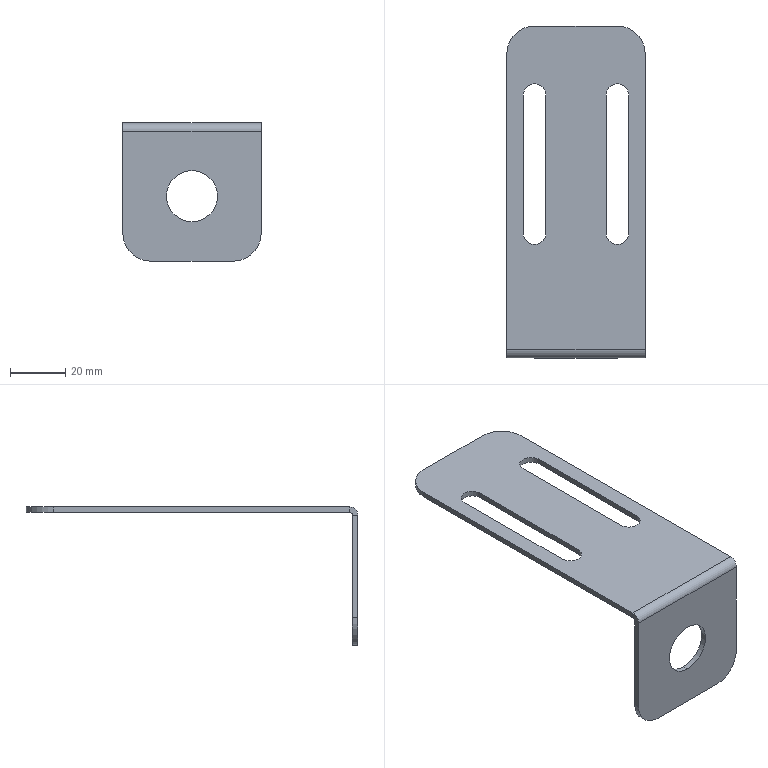Part | SolidWorks | features ICE 2, Fillet 1, FlatPattern 1, SMBaseFlange 1, SheetMetal 1 | 1 solid | 28 faces | box 50 x 120 x 50 mm | volume 14154 mm3 | plane 16 | cylinder 12 | commonest cylinder face diameters 8.2 x4 20 x4 18.5 x2 2 x1 6 x1
STEP:
#1=CARTESIAN_POINT('',(0.,0.,-35.75));
#2=VERTEX_POINT('',#1);
#3=CARTESIAN_POINT('',(0.,0.,-17.25));
#4=VERTEX_POINT('',#3);
#5=CARTESIAN_POINT('',(0.,0.,-26.5));
#6=DIRECTION('',(0.,1.,0.));
#7=DIRECTION('',(0.,0.,-1.));
#8=AXIS2_PLACEMENT_3D('',#5,#6,#7);
#9=CIRCLE('',#8,9.25);
#10=EDGE_CURVE('',#2,#4,#9,.T.);
#11=ORIENTED_EDGE('',*,*,#10,.F.);
#12=CARTESIAN_POINT('',(0.,2.,-35.75));
#13=VERTEX_POINT('',#12);
#14=CARTESIAN_POINT('',(0.,-0.001,-35.75));
#15=DIRECTION('',(0.,1.,0.));
#16=VECTOR('',#15,1000.);
#17=LINE('',#14,#16);
#18=EDGE_CURVE('',#2,#13,#17,.T.);
#19=ORIENTED_EDGE('',*,*,#18,.T.);
#20=CARTESIAN_POINT('',(0.,2.,-17.25));
#21=VERTEX_POINT('',#20);
#22=CARTESIAN_POINT('',(0.,2.,-26.5));
#23=DIRECTION('',(0.,1.,0.));
#24=DIRECTION('',(0.,0.,1.));
#25=AXIS2_PLACEMENT_3D('',#22,#23,#24);
#26=CIRCLE('',#25,9.25);
#27=EDGE_CURVE('',#13,#21,#26,.T.);
#28=ORIENTED_EDGE('',*,*,#27,.T.);
#29=CARTESIAN_POINT('',(0.,-0.001,-17.25));
#30=DIRECTION('',(0.,1.,0.));
#31=VECTOR('',#30,1000.);
#32=LINE('',#29,#31);
#33=EDGE_CURVE('',#4,#21,#32,.T.);
#34=ORIENTED_EDGE('',*,*,#33,.F.);
#35=EDGE_LOOP('',(#11,#19,#28,#34));
#36=FACE_OUTER_BOUND('',#35,.T.);
#37=CARTESIAN_POINT('',(0.,-0.001,-26.5));
#38=DIRECTION('',(0.,1.,0.));
#39=DIRECTION('',(0.,0.,1.));
#40=AXIS2_PLACEMENT_3D('',#37,#38,#39);
#41=CYLINDRICAL_SURFACE('',#40,9.25);
#42=ADVANCED_FACE('',(#36),#41,.F.);
#43=CARTESIAN_POINT('',(25.,3.,0.));
#44=VERTEX_POINT('',#43);
#45=CARTESIAN_POINT('',(25.,3.,-2.));
#46=VERTEX_POINT('',#45);
#47=CARTESIAN_POINT('',(25.,3.,0.));
#48=DIRECTION('',(0.,0.,-1.));
#49=VECTOR('',#48,1000.);
#50=LINE('',#47,#49);
#51=EDGE_CURVE('',#44,#46,#50,.T.);
#52=ORIENTED_EDGE('',*,*,#51,.F.);
#53=CARTESIAN_POINT('',(25.,0.,-3.));
#54=VERTEX_POINT('',#53);
#55=CARTESIAN_POINT('',(25.,3.,-3.));
#56=DIRECTION('',(-1.,0.,0.));
#57=DIRECTION('',(0.,0.,-1.));
#58=AXIS2_PLACEMENT_3D('',#55,#56,#57);
#59=CIRCLE('',#58,3.);
#60=EDGE_CURVE('',#54,#44,#59,.T.);
#61=ORIENTED_EDGE('',*,*,#60,.F.);
#62=CARTESIAN_POINT('',(25.,2.,-3.));
#63=VERTEX_POINT('',#62);
#64=CARTESIAN_POINT('',(25.,2.,-3.));
#65=DIRECTION('',(0.,-1.,0.));
#66=VECTOR('',#65,1000.);
#67=LINE('',#64,#66);
#68=EDGE_CURVE('',#63,#54,#67,.T.);
#69=ORIENTED_EDGE('',*,*,#68,.F.);
#70=CARTESIAN_POINT('',(25.,3.,-3.));
#71=DIRECTION('',(-1.,0.,0.));
#72=DIRECTION('',(0.,0.,-1.));
#73=AXIS2_PLACEMENT_3D('',#70,#71,#72);
#74=CIRCLE('',#73,1.);
#75=EDGE_CURVE('',#63,#46,#74,.T.);
#76=ORIENTED_EDGE('',*,*,#75,.T.);
#77=EDGE_LOOP('',(#52,#61,#69,#76));
#78=FACE_OUTER_BOUND('',#77,.T.);
#79=CARTESIAN_POINT('',(25.,3.,0.));
#80=DIRECTION('',(1.,0.,0.));
#81=DIRECTION('',(0.,0.,-1.));
#82=AXIS2_PLACEMENT_3D('',#79,#80,#81);
#83=PLANE('',#82);
#84=ADVANCED_FACE('',(#78),#83,.T.);
#85=CARTESIAN_POINT('',(25.,110.,-2.));
#86=VERTEX_POINT('',#85);
#87=CARTESIAN_POINT('',(25.,0.,-2.));
#88=DIRECTION('',(0.,1.,0.));
#89=VECTOR('',#88,1000.);
#90=LINE('',#87,#89);
#91=EDGE_CURVE('',#46,#86,#90,.T.);
#92=ORIENTED_EDGE('',*,*,#91,.T.);
#93=CARTESIAN_POINT('',(25.,110.,0.));
#94=VERTEX_POINT('',#93);
#95=CARTESIAN_POINT('',(25.,110.,-3.));
#96=DIRECTION('',(0.,0.,1.));
#97=VECTOR('',#96,1000.);
#98=LINE('',#95,#97);
#99=EDGE_CURVE('',#86,#94,#98,.T.);
#100=ORIENTED_EDGE('',*,*,#99,.T.);
#101=CARTESIAN_POINT('',(25.,0.,0.));
#102=DIRECTION('',(0.,1.,0.));
#103=VECTOR('',#102,1000.);
#104=LINE('',#101,#103);
#105=EDGE_CURVE('',#44,#94,#104,.T.);
#106=ORIENTED_EDGE('',*,*,#105,.F.);
#107=ORIENTED_EDGE('',*,*,#51,.T.);
#108=EDGE_LOOP('',(#92,#100,#106,#107));
#109=FACE_OUTER_BOUND('',#108,.T.);
#110=CARTESIAN_POINT('',(25.,2.,-3.));
#111=DIRECTION('',(1.,0.,0.));
#112=DIRECTION('',(0.,0.,-1.));
#113=AXIS2_PLACEMENT_3D('',#110,#111,#112);
#114=PLANE('',#113);
#115=ADVANCED_FACE('',(#109),#114,.T.);
#116=CARTESIAN_POINT('',(-25.,0.,-3.));
#117=VERTEX_POINT('',#116);
#118=CARTESIAN_POINT('',(-25.,2.,-3.));
#119=VERTEX_POINT('',#118);
#120=CARTESIAN_POINT('',(-25.,0.,-3.));
#121=DIRECTION('',(0.,1.,0.));
#122=VECTOR('',#121,1000.);
#123=LINE('',#120,#122);
#124=EDGE_CURVE('',#117,#119,#123,.T.);
#125=ORIENTED_EDGE('',*,*,#124,.F.);
#126=CARTESIAN_POINT('',(-25.,3.,0.));
#127=VERTEX_POINT('',#126);
#128=CARTESIAN_POINT('',(-25.,3.,-3.));
#129=DIRECTION('',(-1.,0.,0.));
#130=DIRECTION('',(0.,0.,-1.));
#131=AXIS2_PLACEMENT_3D('',#128,#129,#130);
#132=CIRCLE('',#131,3.);
#133=EDGE_CURVE('',#117,#127,#132,.T.);
#134=ORIENTED_EDGE('',*,*,#133,.T.);
#135=CARTESIAN_POINT('',(-25.,3.,-2.));
#136=VERTEX_POINT('',#135);
#137=CARTESIAN_POINT('',(-25.,3.,-2.));
#138=DIRECTION('',(0.,0.,1.));
#139=VECTOR('',#138,1000.);
#140=LINE('',#137,#139);
#141=EDGE_CURVE('',#136,#127,#140,.T.);
#142=ORIENTED_EDGE('',*,*,#141,.F.);
#143=CARTESIAN_POINT('',(-25.,3.,-3.));
#144=DIRECTION('',(-1.,0.,0.));
#145=DIRECTION('',(0.,0.,-1.));
#146=AXIS2_PLACEMENT_3D('',#143,#144,#145);
#147=CIRCLE('',#146,1.);
#148=EDGE_CURVE('',#119,#136,#147,.T.);
#149=ORIENTED_EDGE('',*,*,#148,.F.);
#150=EDGE_LOOP('',(#125,#134,#142,#149));
#151=FACE_OUTER_BOUND('',#150,.T.);
#152=CARTESIAN_POINT('',(-25.,0.,-3.));
#153=DIRECTION('',(-1.,0.,0.));
#154=DIRECTION('',(0.,0.,1.));
#155=AXIS2_PLACEMENT_3D('',#152,#153,#154);
#156=PLANE('',#155);
#157=ADVANCED_FACE('',(#151),#156,.T.);
#158=CARTESIAN_POINT('',(-25.,2.,-40.));
#159=VERTEX_POINT('',#158);
#160=CARTESIAN_POINT('',(-25.,2.,0.));
#161=DIRECTION('',(0.,0.,1.));
#162=VECTOR('',#161,1000.);
#163=LINE('',#160,#162);
#164=EDGE_CURVE('',#159,#119,#163,.T.);
#165=ORIENTED_EDGE('',*,*,#164,.F.);
#166=CARTESIAN_POINT('',(-25.,0.,-40.));
#167=VERTEX_POINT('',#166);
#168=CARTESIAN_POINT('',(-25.,3.,-40.));
#169=DIRECTION('',(0.,-1.,0.));
#170=VECTOR('',#169,1000.);
#171=LINE('',#168,#170);
#172=EDGE_CURVE('',#159,#167,#171,.T.);
#173=ORIENTED_EDGE('',*,*,#172,.T.);
#174=CARTESIAN_POINT('',(-25.,0.,0.));
#175=DIRECTION('',(0.,0.,1.));
#176=VECTOR('',#175,1000.);
#177=LINE('',#174,#176);
#178=EDGE_CURVE('',#167,#117,#177,.T.);
#179=ORIENTED_EDGE('',*,*,#178,.T.);
#180=ORIENTED_EDGE('',*,*,#124,.T.);
#181=EDGE_LOOP('',(#165,#173,#179,#180));
#182=FACE_OUTER_BOUND('',#181,.T.);
#183=CARTESIAN_POINT('',(-25.,3.,-2.));
#184=DIRECTION('',(-1.,0.,0.));
#185=DIRECTION('',(0.,0.,1.));
#186=AXIS2_PLACEMENT_3D('',#183,#184,#185);
#187=PLANE('',#186);
#188=ADVANCED_FACE('',(#182),#187,.T.);
#189=CARTESIAN_POINT('',(-19.1,45.,-2.));
#190=VERTEX_POINT('',#189);
#191=CARTESIAN_POINT('',(-19.1,95.,-2.));
#192=VERTEX_POINT('',#191);
#193=CARTESIAN_POINT('',(-19.1,45.,-2.));
#194=DIRECTION('',(0.,1.,0.));
#195=VECTOR('',#194,1000.);
#196=LINE('',#193,#195);
#197=EDGE_CURVE('',#190,#192,#196,.T.);
#198=ORIENTED_EDGE('',*,*,#197,.F.);
#199=CARTESIAN_POINT('',(-10.9,45.,-2.));
#200=VERTEX_POINT('',#199);
#201=CARTESIAN_POINT('',(-15.,45.,-2.));
#202=DIRECTION('',(0.,0.,-1.));
#203=DIRECTION('',(-1.,0.,0.));
#204=AXIS2_PLACEMENT_3D('',#201,#202,#203);
#205=CIRCLE('',#204,4.1);
#206=EDGE_CURVE('',#200,#190,#205,.T.);
#207=ORIENTED_EDGE('',*,*,#206,.F.);
#208=CARTESIAN_POINT('',(-10.9,95.,-2.));
#209=VERTEX_POINT('',#208);
#210=CARTESIAN_POINT('',(-10.9,45.,-2.));
#211=DIRECTION('',(0.,-1.,0.));
#212=VECTOR('',#211,1000.);
#213=LINE('',#210,#212);
#214=EDGE_CURVE('',#209,#200,#213,.T.);
#215=ORIENTED_EDGE('',*,*,#214,.F.);
#216=CARTESIAN_POINT('',(-15.,95.,-2.));
#217=DIRECTION('',(0.,0.,-1.));
#218=DIRECTION('',(-1.,0.,0.));
#219=AXIS2_PLACEMENT_3D('',#216,#217,#218);
#220=CIRCLE('',#219,4.1);
#221=EDGE_CURVE('',#192,#209,#220,.T.);
#222=ORIENTED_EDGE('',*,*,#221,.F.);
#223=EDGE_LOOP('',(#198,#207,#215,#222));
#224=FACE_BOUND('',#223,.T.);
#225=CARTESIAN_POINT('',(10.9,45.,-2.));
#226=VERTEX_POINT('',#225);
#227=CARTESIAN_POINT('',(10.9,95.,-2.));
#228=VERTEX_POINT('',#227);
#229=CARTESIAN_POINT('',(10.9,45.,-2.));
#230=DIRECTION('',(0.,1.,0.));
#231=VECTOR('',#230,1000.);
#232=LINE('',#229,#231);
#233=EDGE_CURVE('',#226,#228,#232,.T.);
#234=ORIENTED_EDGE('',*,*,#233,.F.);
#235=CARTESIAN_POINT('',(19.1,45.,-2.));
#236=VERTEX_POINT('',#235);
#237=CARTESIAN_POINT('',(15.,45.,-2.));
#238=DIRECTION('',(0.,0.,-1.));
#239=DIRECTION('',(1.,0.,0.));
#240=AXIS2_PLACEMENT_3D('',#237,#238,#239);
#241=CIRCLE('',#240,4.1);
#242=EDGE_CURVE('',#236,#226,#241,.T.);
#243=ORIENTED_EDGE('',*,*,#242,.F.);
#244=CARTESIAN_POINT('',(19.1,95.,-2.));
#245=VERTEX_POINT('',#244);
#246=CARTESIAN_POINT('',(19.1,45.,-2.));
#247=DIRECTION('',(0.,-1.,0.));
#248=VECTOR('',#247,1000.);
#249=LINE('',#246,#248);
#250=EDGE_CURVE('',#245,#236,#249,.T.);
#251=ORIENTED_EDGE('',*,*,#250,.F.);
#252=CARTESIAN_POINT('',(15.,95.,-2.));
#253=DIRECTION('',(0.,0.,-1.));
#254=DIRECTION('',(1.,0.,0.));
#255=AXIS2_PLACEMENT_3D('',#252,#253,#254);
#256=CIRCLE('',#255,4.1);
#257=EDGE_CURVE('',#228,#245,#256,.T.);
#258=ORIENTED_EDGE('',*,*,#257,.F.);
#259=EDGE_LOOP('',(#234,#243,#251,#258));
#260=FACE_BOUND('',#259,.T.);
#261=CARTESIAN_POINT('',(15.,120.,-2.));
#262=VERTEX_POINT('',#261);
#263=CARTESIAN_POINT('',(-15.,120.,-2.));
#264=VERTEX_POINT('',#263);
#265=CARTESIAN_POINT('',(25.,120.,-2.));
#266=DIRECTION('',(-1.,0.,0.));
#267=VECTOR('',#266,1000.);
#268=LINE('',#265,#267);
#269=EDGE_CURVE('',#262,#264,#268,.T.);
#270=ORIENTED_EDGE('',*,*,#269,.F.);
#271=CARTESIAN_POINT('',(15.,110.,-2.));
#272=DIRECTION('',(0.,0.,-1.));
#273=DIRECTION('',(1.,0.,0.));
#274=AXIS2_PLACEMENT_3D('',#271,#272,#273);
#275=CIRCLE('',#274,10.);
#276=EDGE_CURVE('',#262,#86,#275,.T.);
#277=ORIENTED_EDGE('',*,*,#276,.T.);
#278=ORIENTED_EDGE('',*,*,#91,.F.);
#279=CARTESIAN_POINT('',(25.,3.,-2.));
#280=DIRECTION('',(-1.,0.,0.));
#281=VECTOR('',#280,1000.);
#282=LINE('',#279,#281);
#283=EDGE_CURVE('',#46,#136,#282,.T.);
#284=ORIENTED_EDGE('',*,*,#283,.T.);
#285=CARTESIAN_POINT('',(-25.,110.,-2.));
#286=VERTEX_POINT('',#285);
#287=CARTESIAN_POINT('',(-25.,0.,-2.));
#288=DIRECTION('',(0.,1.,0.));
#289=VECTOR('',#288,1000.);
#290=LINE('',#287,#289);
#291=EDGE_CURVE('',#136,#286,#290,.T.);
#292=ORIENTED_EDGE('',*,*,#291,.T.);
#293=CARTESIAN_POINT('',(-15.,110.,-2.));
#294=DIRECTION('',(0.,0.,-1.));
#295=DIRECTION('',(1.,0.,0.));
#296=AXIS2_PLACEMENT_3D('',#293,#294,#295);
#297=CIRCLE('',#296,10.);
#298=EDGE_CURVE('',#286,#264,#297,.T.);
#299=ORIENTED_EDGE('',*,*,#298,.T.);
#300=EDGE_LOOP('',(#270,#277,#278,#284,#292,#299));
#301=FACE_OUTER_BOUND('',#300,.T.);
#302=CARTESIAN_POINT('',(25.,0.,-2.));
#303=DIRECTION('',(0.,0.,1.));
#304=DIRECTION('',(1.,0.,0.));
#305=AXIS2_PLACEMENT_3D('',#302,#303,#304);
#306=PLANE('',#305);
#307=ADVANCED_FACE('',(#224,#260,#301),#306,.F.);
#308=CARTESIAN_POINT('',(15.,120.,0.));
#309=VERTEX_POINT('',#308);
#310=CARTESIAN_POINT('',(-15.,120.,0.));
#311=VERTEX_POINT('',#310);
#312=CARTESIAN_POINT('',(25.,120.,0.));
#313=DIRECTION('',(-1.,0.,0.));
#314=VECTOR('',#313,1000.);
#315=LINE('',#312,#314);
#316=EDGE_CURVE('',#309,#311,#315,.T.);
#317=ORIENTED_EDGE('',*,*,#316,.F.);
#318=CARTESIAN_POINT('',(15.,120.,0.));
#319=DIRECTION('',(0.,0.,-1.));
#320=VECTOR('',#319,1000.);
#321=LINE('',#318,#320);
#322=EDGE_CURVE('',#309,#262,#321,.T.);
#323=ORIENTED_EDGE('',*,*,#322,.T.);
#324=ORIENTED_EDGE('',*,*,#269,.T.);
#325=CARTESIAN_POINT('',(-15.,120.,0.));
#326=DIRECTION('',(0.,0.,1.));
#327=VECTOR('',#326,1000.);
#328=LINE('',#325,#327);
#329=EDGE_CURVE('',#264,#311,#328,.T.);
#330=ORIENTED_EDGE('',*,*,#329,.T.);
#331=EDGE_LOOP('',(#317,#323,#324,#330));
#332=FACE_OUTER_BOUND('',#331,.T.);
#333=CARTESIAN_POINT('',(25.,120.,0.));
#334=DIRECTION('',(0.,1.,0.));
#335=DIRECTION('',(0.,0.,1.));
#336=AXIS2_PLACEMENT_3D('',#333,#334,#335);
#337=PLANE('',#336);
#338=ADVANCED_FACE('',(#332),#337,.T.);
#339=CARTESIAN_POINT('',(-10.9,45.,0.));
#340=VERTEX_POINT('',#339);
#341=CARTESIAN_POINT('',(-19.1,45.,0.));
#342=VERTEX_POINT('',#341);
#343=CARTESIAN_POINT('',(-15.,45.,0.));
#344=DIRECTION('',(0.,0.,-1.));
#345=DIRECTION('',(1.,0.,0.));
#346=AXIS2_PLACEMENT_3D('',#343,#344,#345);
#347=CIRCLE('',#346,4.1);
#348=EDGE_CURVE('',#340,#342,#347,.T.);
#349=ORIENTED_EDGE('',*,*,#348,.T.);
#350=CARTESIAN_POINT('',(-19.1,95.,0.));
#351=VERTEX_POINT('',#350);
#352=CARTESIAN_POINT('',(-19.1,45.,0.));
#353=DIRECTION('',(0.,1.,0.));
#354=VECTOR('',#353,1000.);
#355=LINE('',#352,#354);
#356=EDGE_CURVE('',#342,#351,#355,.T.);
#357=ORIENTED_EDGE('',*,*,#356,.T.);
#358=CARTESIAN_POINT('',(-10.9,95.,0.));
#359=VERTEX_POINT('',#358);
#360=CARTESIAN_POINT('',(-15.,95.,0.));
#361=DIRECTION('',(0.,0.,-1.));
#362=DIRECTION('',(1.,0.,0.));
#363=AXIS2_PLACEMENT_3D('',#360,#361,#362);
#364=CIRCLE('',#363,4.1);
#365=EDGE_CURVE('',#351,#359,#364,.T.);
#366=ORIENTED_EDGE('',*,*,#365,.T.);
#367=CARTESIAN_POINT('',(-10.9,45.,0.));
#368=DIRECTION('',(0.,-1.,0.));
#369=VECTOR('',#368,1000.);
#370=LINE('',#367,#369);
#371=EDGE_CURVE('',#359,#340,#370,.T.);
#372=ORIENTED_EDGE('',*,*,#371,.T.);
#373=EDGE_LOOP('',(#349,#357,#366,#372));
#374=FACE_BOUND('',#373,.T.);
#375=CARTESIAN_POINT('',(19.1,45.,0.));
#376=VERTEX_POINT('',#375);
#377=CARTESIAN_POINT('',(10.9,45.,0.));
#378=VERTEX_POINT('',#377);
#379=CARTESIAN_POINT('',(15.,45.,0.));
#380=DIRECTION('',(0.,0.,-1.));
#381=DIRECTION('',(1.,0.,0.));
#382=AXIS2_PLACEMENT_3D('',#379,#380,#381);
#383=CIRCLE('',#382,4.1);
#384=EDGE_CURVE('',#376,#378,#383,.T.);
#385=ORIENTED_EDGE('',*,*,#384,.T.);
#386=CARTESIAN_POINT('',(10.9,95.,0.));
#387=VERTEX_POINT('',#386);
#388=CARTESIAN_POINT('',(10.9,45.,0.));
#389=DIRECTION('',(0.,1.,0.));
#390=VECTOR('',#389,1000.);
#391=LINE('',#388,#390);
#392=EDGE_CURVE('',#378,#387,#391,.T.);
#393=ORIENTED_EDGE('',*,*,#392,.T.);
#394=CARTESIAN_POINT('',(19.1,95.,0.));
#395=VERTEX_POINT('',#394);
#396=CARTESIAN_POINT('',(15.,95.,0.));
#397=DIRECTION('',(0.,0.,-1.));
#398=DIRECTION('',(1.,0.,0.));
#399=AXIS2_PLACEMENT_3D('',#396,#397,#398);
#400=CIRCLE('',#399,4.1);
#401=EDGE_CURVE('',#387,#395,#400,.T.);
#402=ORIENTED_EDGE('',*,*,#401,.T.);
#403=CARTESIAN_POINT('',(19.1,45.,0.));
#404=DIRECTION('',(0.,-1.,0.));
#405=VECTOR('',#404,1000.);
#406=LINE('',#403,#405);
#407=EDGE_CURVE('',#395,#376,#406,.T.);
#408=ORIENTED_EDGE('',*,*,#407,.T.);
#409=EDGE_LOOP('',(#385,#393,#402,#408));
#410=FACE_BOUND('',#409,.T.);
#411=ORIENTED_EDGE('',*,*,#105,.T.);
#412=CARTESIAN_POINT('',(15.,110.,0.));
#413=DIRECTION('',(0.,0.,1.));
#414=DIRECTION('',(1.,0.,0.));
#415=AXIS2_PLACEMENT_3D('',#412,#413,#414);
#416=CIRCLE('',#415,10.);
#417=EDGE_CURVE('',#94,#309,#416,.T.);
#418=ORIENTED_EDGE('',*,*,#417,.T.);
#419=ORIENTED_EDGE('',*,*,#316,.T.);
#420=CARTESIAN_POINT('',(-25.,110.,0.));
#421=VERTEX_POINT('',#420);
#422=CARTESIAN_POINT('',(-15.,110.,0.));
#423=DIRECTION('',(0.,0.,1.));
#424=DIRECTION('',(1.,0.,0.));
#425=AXIS2_PLACEMENT_3D('',#422,#423,#424);
#426=CIRCLE('',#425,10.);
#427=EDGE_CURVE('',#311,#421,#426,.T.);
#428=ORIENTED_EDGE('',*,*,#427,.T.);
#429=CARTESIAN_POINT('',(-25.,0.,0.));
#430=DIRECTION('',(0.,1.,0.));
#431=VECTOR('',#430,1000.);
#432=LINE('',#429,#431);
#433=EDGE_CURVE('',#127,#421,#432,.T.);
#434=ORIENTED_EDGE('',*,*,#433,.F.);
#435=CARTESIAN_POINT('',(25.,3.,0.));
#436=DIRECTION('',(-1.,0.,0.));
#437=VECTOR('',#436,1000.);
#438=LINE('',#435,#437);
#439=EDGE_CURVE('',#44,#127,#438,.T.);
#440=ORIENTED_EDGE('',*,*,#439,.F.);
#441=EDGE_LOOP('',(#411,#418,#419,#428,#434,#440));
#442=FACE_OUTER_BOUND('',#441,.T.);
#443=CARTESIAN_POINT('',(25.,0.,0.));
#444=DIRECTION('',(0.,0.,1.));
#445=DIRECTION('',(1.,0.,0.));
#446=AXIS2_PLACEMENT_3D('',#443,#444,#445);
#447=PLANE('',#446);
#448=ADVANCED_FACE('',(#374,#410,#442),#447,.T.);
#449=ORIENTED_EDGE('',*,*,#133,.F.);
#450=CARTESIAN_POINT('',(25.,0.,-3.));
#451=DIRECTION('',(-1.,0.,0.));
#452=VECTOR('',#451,1000.);
#453=LINE('',#450,#452);
#454=EDGE_CURVE('',#54,#117,#453,.T.);
#455=ORIENTED_EDGE('',*,*,#454,.F.);
#456=ORIENTED_EDGE('',*,*,#60,.T.);
#457=ORIENTED_EDGE('',*,*,#439,.T.);
#458=EDGE_LOOP('',(#449,#455,#456,#457));
#459=FACE_OUTER_BOUND('',#458,.T.);
#460=CARTESIAN_POINT('',(25.,3.,-3.));
#461=DIRECTION('',(-1.,0.,0.));
#462=DIRECTION('',(0.,0.,1.));
#463=AXIS2_PLACEMENT_3D('',#460,#461,#462);
#464=CYLINDRICAL_SURFACE('',#463,3.);
#465=ADVANCED_FACE('',(#459),#464,.T.);
#466=CARTESIAN_POINT('',(0.,0.,-26.5));
#467=DIRECTION('',(0.,1.,0.));
#468=DIRECTION('',(0.,0.,-1.));
#469=AXIS2_PLACEMENT_3D('',#466,#467,#468);
#470=CIRCLE('',#469,9.25);
#471=EDGE_CURVE('',#4,#2,#470,.T.);
#472=ORIENTED_EDGE('',*,*,#471,.T.);
#473=ORIENTED_EDGE('',*,*,#10,.T.);
#474=EDGE_LOOP('',(#472,#473));
#475=FACE_BOUND('',#474,.T.);
#476=CARTESIAN_POINT('',(15.,0.,-50.));
#477=VERTEX_POINT('',#476);
#478=CARTESIAN_POINT('',(-15.,0.,-50.));
#479=VERTEX_POINT('',#478);
#480=CARTESIAN_POINT('',(25.,0.,-50.));
#481=DIRECTION('',(-1.,0.,0.));
#482=VECTOR('',#481,1000.);
#483=LINE('',#480,#482);
#484=EDGE_CURVE('',#477,#479,#483,.T.);
#485=ORIENTED_EDGE('',*,*,#484,.F.);
#486=CARTESIAN_POINT('',(25.,0.,-40.));
#487=VERTEX_POINT('',#486);
#488=CARTESIAN_POINT('',(15.,0.,-40.));
#489=DIRECTION('',(0.,-1.,0.));
#490=DIRECTION('',(0.,0.,-1.));
#491=AXIS2_PLACEMENT_3D('',#488,#489,#490);
#492=CIRCLE('',#491,10.);
#493=EDGE_CURVE('',#477,#487,#492,.T.);
#494=ORIENTED_EDGE('',*,*,#493,.T.);
#495=CARTESIAN_POINT('',(25.,0.,0.));
#496=DIRECTION('',(0.,0.,1.));
#497=VECTOR('',#496,1000.);
#498=LINE('',#495,#497);
#499=EDGE_CURVE('',#487,#54,#498,.T.);
#500=ORIENTED_EDGE('',*,*,#499,.T.);
#501=ORIENTED_EDGE('',*,*,#454,.T.);
#502=ORIENTED_EDGE('',*,*,#178,.F.);
#503=CARTESIAN_POINT('',(-15.,0.,-40.));
#504=DIRECTION('',(0.,-1.,0.));
#505=DIRECTION('',(0.,0.,-1.));
#506=AXIS2_PLACEMENT_3D('',#503,#504,#505);
#507=CIRCLE('',#506,10.);
#508=EDGE_CURVE('',#167,#479,#507,.T.);
#509=ORIENTED_EDGE('',*,*,#508,.T.);
#510=EDGE_LOOP('',(#485,#494,#500,#501,#502,#509));
#511=FACE_OUTER_BOUND('',#510,.T.);
#512=CARTESIAN_POINT('',(25.,0.,0.));
#513=DIRECTION('',(0.,-1.,0.));
#514=DIRECTION('',(0.,0.,-1.));
#515=AXIS2_PLACEMENT_3D('',#512,#513,#514);
#516=PLANE('',#515);
#517=ADVANCED_FACE('',(#475,#511),#516,.T.);
#518=CARTESIAN_POINT('',(15.,2.,-50.));
#519=VERTEX_POINT('',#518);
#520=CARTESIAN_POINT('',(-15.,2.,-50.));
#521=VERTEX_POINT('',#520);
#522=CARTESIAN_POINT('',(25.,2.,-50.));
#523=DIRECTION('',(-1.,0.,0.));
#524=VECTOR('',#523,1000.);
#525=LINE('',#522,#524);
#526=EDGE_CURVE('',#519,#521,#525,.T.);
#527=ORIENTED_EDGE('',*,*,#526,.F.);
#528=CARTESIAN_POINT('',(15.,2.,-50.));
#529=DIRECTION('',(0.,-1.,0.));
#530=VECTOR('',#529,1000.);
#531=LINE('',#528,#530);
#532=EDGE_CURVE('',#519,#477,#531,.T.);
#533=ORIENTED_EDGE('',*,*,#532,.T.);
#534=ORIENTED_EDGE('',*,*,#484,.T.);
#535=CARTESIAN_POINT('',(-15.,2.,-50.));
#536=DIRECTION('',(0.,1.,0.));
#537=VECTOR('',#536,1000.);
#538=LINE('',#535,#537);
#539=EDGE_CURVE('',#479,#521,#538,.T.);
#540=ORIENTED_EDGE('',*,*,#539,.T.);
#541=EDGE_LOOP('',(#527,#533,#534,#540));
#542=FACE_OUTER_BOUND('',#541,.T.);
#543=CARTESIAN_POINT('',(25.,2.,-50.));
#544=DIRECTION('',(0.,0.,-1.));
#545=DIRECTION('',(-1.,0.,0.));
#546=AXIS2_PLACEMENT_3D('',#543,#544,#545);
#547=PLANE('',#546);
#548=ADVANCED_FACE('',(#542),#547,.T.);
#549=CARTESIAN_POINT('',(0.,2.,-26.5));
#550=DIRECTION('',(0.,1.,0.));
#551=DIRECTION('',(0.,0.,1.));
#552=AXIS2_PLACEMENT_3D('',#549,#550,#551);
#553=CIRCLE('',#552,9.25);
#554=EDGE_CURVE('',#21,#13,#553,.T.);
#555=ORIENTED_EDGE('',*,*,#554,.F.);
#556=ORIENTED_EDGE('',*,*,#27,.F.);
#557=EDGE_LOOP('',(#555,#556));
#558=FACE_BOUND('',#557,.T.);
#559=CARTESIAN_POINT('',(25.,2.,-40.));
#560=VERTEX_POINT('',#559);
#561=CARTESIAN_POINT('',(25.,2.,0.));
#562=DIRECTION('',(0.,0.,1.));
#563=VECTOR('',#562,1000.);
#564=LINE('',#561,#563);
#565=EDGE_CURVE('',#560,#63,#564,.T.);
#566=ORIENTED_EDGE('',*,*,#565,.F.);
#567=CARTESIAN_POINT('',(15.,2.,-40.));
#568=DIRECTION('',(0.,1.,0.));
#569=DIRECTION('',(0.,0.,-1.));
#570=AXIS2_PLACEMENT_3D('',#567,#568,#569);
#571=CIRCLE('',#570,10.);
#572=EDGE_CURVE('',#560,#519,#571,.T.);
#573=ORIENTED_EDGE('',*,*,#572,.T.);
#574=ORIENTED_EDGE('',*,*,#526,.T.);
#575=CARTESIAN_POINT('',(-15.,2.,-40.));
#576=DIRECTION('',(0.,1.,0.));
#577=DIRECTION('',(0.,0.,-1.));
#578=AXIS2_PLACEMENT_3D('',#575,#576,#577);
#579=CIRCLE('',#578,10.);
#580=EDGE_CURVE('',#521,#159,#579,.T.);
#581=ORIENTED_EDGE('',*,*,#580,.T.);
#582=ORIENTED_EDGE('',*,*,#164,.T.);
#583=CARTESIAN_POINT('',(25.,2.,-3.));
#584=DIRECTION('',(-1.,0.,0.));
#585=VECTOR('',#584,1000.);
#586=LINE('',#583,#585);
#587=EDGE_CURVE('',#63,#119,#586,.T.);
#588=ORIENTED_EDGE('',*,*,#587,.F.);
#589=EDGE_LOOP('',(#566,#573,#574,#581,#582,#588));
#590=FACE_OUTER_BOUND('',#589,.T.);
#591=CARTESIAN_POINT('',(25.,2.,0.));
#592=DIRECTION('',(0.,-1.,0.));
#593=DIRECTION('',(0.,0.,-1.));
#594=AXIS2_PLACEMENT_3D('',#591,#592,#593);
#595=PLANE('',#594);
#596=ADVANCED_FACE('',(#558,#590),#595,.F.);
#597=ORIENTED_EDGE('',*,*,#148,.T.);
#598=ORIENTED_EDGE('',*,*,#283,.F.);
#599=ORIENTED_EDGE('',*,*,#75,.F.);
#600=ORIENTED_EDGE('',*,*,#587,.T.);
#601=EDGE_LOOP('',(#597,#598,#599,#600));
#602=FACE_OUTER_BOUND('',#601,.T.);
#603=CARTESIAN_POINT('',(25.,3.,-3.));
#604=DIRECTION('',(-1.,0.,0.));
#605=DIRECTION('',(0.,0.,1.));
#606=AXIS2_PLACEMENT_3D('',#603,#604,#605);
#607=CYLINDRICAL_SURFACE('',#606,1.);
#608=ADVANCED_FACE('',(#602),#607,.F.);
#609=ORIENTED_EDGE('',*,*,#499,.F.);
#610=CARTESIAN_POINT('',(25.,3.,-40.));
#611=DIRECTION('',(0.,1.,0.));
#612=VECTOR('',#611,1000.);
#613=LINE('',#610,#612);
#614=EDGE_CURVE('',#487,#560,#613,.T.);
#615=ORIENTED_EDGE('',*,*,#614,.T.);
#616=ORIENTED_EDGE('',*,*,#565,.T.);
#617=ORIENTED_EDGE('',*,*,#68,.T.);
#618=EDGE_LOOP('',(#609,#615,#616,#617));
#619=FACE_OUTER_BOUND('',#618,.T.);
#620=CARTESIAN_POINT('',(25.,3.,-3.));
#621=DIRECTION('',(1.,0.,0.));
#622=DIRECTION('',(0.,0.,-1.));
#623=AXIS2_PLACEMENT_3D('',#620,#621,#622);
#624=PLANE('',#623);
#625=ADVANCED_FACE('',(#619),#624,.T.);
#626=ORIENTED_EDGE('',*,*,#433,.T.);
#627=CARTESIAN_POINT('',(-25.,110.,-2.));
#628=DIRECTION('',(0.,0.,-1.));
#629=VECTOR('',#628,1000.);
#630=LINE('',#627,#629);
#631=EDGE_CURVE('',#421,#286,#630,.T.);
#632=ORIENTED_EDGE('',*,*,#631,.T.);
#633=ORIENTED_EDGE('',*,*,#291,.F.);
#634=ORIENTED_EDGE('',*,*,#141,.T.);
#635=EDGE_LOOP('',(#626,#632,#633,#634));
#636=FACE_OUTER_BOUND('',#635,.T.);
#637=CARTESIAN_POINT('',(-25.,3.,-3.));
#638=DIRECTION('',(1.,0.,0.));
#639=DIRECTION('',(0.,0.,-1.));
#640=AXIS2_PLACEMENT_3D('',#637,#638,#639);
#641=PLANE('',#640);
#642=ADVANCED_FACE('',(#636),#641,.F.);
#643=ORIENTED_EDGE('',*,*,#18,.F.);
#644=ORIENTED_EDGE('',*,*,#471,.F.);
#645=ORIENTED_EDGE('',*,*,#33,.T.);
#646=ORIENTED_EDGE('',*,*,#554,.T.);
#647=EDGE_LOOP('',(#643,#644,#645,#646));
#648=FACE_OUTER_BOUND('',#647,.T.);
#649=CARTESIAN_POINT('',(0.,-0.001,-26.5));
#650=DIRECTION('',(0.,1.,0.));
#651=DIRECTION('',(0.,0.,1.));
#652=AXIS2_PLACEMENT_3D('',#649,#650,#651);
#653=CYLINDRICAL_SURFACE('',#652,9.25);
#654=ADVANCED_FACE('',(#648),#653,.F.);
#655=ORIENTED_EDGE('',*,*,#417,.F.);
#656=ORIENTED_EDGE('',*,*,#99,.F.);
#657=ORIENTED_EDGE('',*,*,#276,.F.);
#658=ORIENTED_EDGE('',*,*,#322,.F.);
#659=EDGE_LOOP('',(#655,#656,#657,#658));
#660=FACE_OUTER_BOUND('',#659,.T.);
#661=CARTESIAN_POINT('',(15.,110.,0.));
#662=DIRECTION('',(0.,0.,-1.));
#663=DIRECTION('',(-1.,0.,0.));
#664=AXIS2_PLACEMENT_3D('',#661,#662,#663);
#665=CYLINDRICAL_SURFACE('',#664,10.);
#666=ADVANCED_FACE('',(#660),#665,.T.);
#667=ORIENTED_EDGE('',*,*,#427,.F.);
#668=ORIENTED_EDGE('',*,*,#329,.F.);
#669=ORIENTED_EDGE('',*,*,#298,.F.);
#670=ORIENTED_EDGE('',*,*,#631,.F.);
#671=EDGE_LOOP('',(#667,#668,#669,#670));
#672=FACE_OUTER_BOUND('',#671,.T.);
#673=CARTESIAN_POINT('',(-15.,110.,-3.));
#674=DIRECTION('',(0.,0.,1.));
#675=DIRECTION('',(1.,0.,0.));
#676=AXIS2_PLACEMENT_3D('',#673,#674,#675);
#677=CYLINDRICAL_SURFACE('',#676,10.);
#678=ADVANCED_FACE('',(#672),#677,.T.);
#679=ORIENTED_EDGE('',*,*,#572,.F.);
#680=ORIENTED_EDGE('',*,*,#614,.F.);
#681=ORIENTED_EDGE('',*,*,#493,.F.);
#682=ORIENTED_EDGE('',*,*,#532,.F.);
#683=EDGE_LOOP('',(#679,#680,#681,#682));
#684=FACE_OUTER_BOUND('',#683,.T.);
#685=CARTESIAN_POINT('',(15.,2.,-40.));
#686=DIRECTION('',(0.,-1.,0.));
#687=DIRECTION('',(0.,0.,-1.));
#688=AXIS2_PLACEMENT_3D('',#685,#686,#687);
#689=CYLINDRICAL_SURFACE('',#688,10.);
#690=ADVANCED_FACE('',(#684),#689,.T.);
#691=ORIENTED_EDGE('',*,*,#580,.F.);
#692=ORIENTED_EDGE('',*,*,#539,.F.);
#693=ORIENTED_EDGE('',*,*,#508,.F.);
#694=ORIENTED_EDGE('',*,*,#172,.F.);
#695=EDGE_LOOP('',(#691,#692,#693,#694));
#696=FACE_OUTER_BOUND('',#695,.T.);
#697=CARTESIAN_POINT('',(-15.,3.,-40.));
#698=DIRECTION('',(0.,-1.,0.));
#699=DIRECTION('',(0.,0.,-1.));
#700=AXIS2_PLACEMENT_3D('',#697,#698,#699);
#701=CYLINDRICAL_SURFACE('',#700,10.);
#702=ADVANCED_FACE('',(#696),#701,.T.);
#703=CARTESIAN_POINT('',(19.1,45.,0.001));
#704=DIRECTION('',(0.,0.,-1.));
#705=VECTOR('',#704,1000.);
#706=LINE('',#703,#705);
#707=EDGE_CURVE('',#376,#236,#706,.T.);
#708=ORIENTED_EDGE('',*,*,#707,.T.);
#709=ORIENTED_EDGE('',*,*,#242,.T.);
#710=CARTESIAN_POINT('',(10.9,45.,0.001));
#711=DIRECTION('',(0.,0.,-1.));
#712=VECTOR('',#711,1000.);
#713=LINE('',#710,#712);
#714=EDGE_CURVE('',#378,#226,#713,.T.);
#715=ORIENTED_EDGE('',*,*,#714,.F.);
#716=ORIENTED_EDGE('',*,*,#384,.F.);
#717=EDGE_LOOP('',(#708,#709,#715,#716));
#718=FACE_OUTER_BOUND('',#717,.T.);
#719=CARTESIAN_POINT('',(15.,45.,0.001));
#720=DIRECTION('',(0.,0.,-1.));
#721=DIRECTION('',(-1.,0.,0.));
#722=AXIS2_PLACEMENT_3D('',#719,#720,#721);
#723=CYLINDRICAL_SURFACE('',#722,4.1);
#724=ADVANCED_FACE('',(#718),#723,.F.);
#725=CARTESIAN_POINT('',(19.1,95.,0.001));
#726=DIRECTION('',(0.,0.,-1.));
#727=VECTOR('',#726,1000.);
#728=LINE('',#725,#727);
#729=EDGE_CURVE('',#395,#245,#728,.T.);
#730=ORIENTED_EDGE('',*,*,#729,.T.);
#731=ORIENTED_EDGE('',*,*,#250,.T.);
#732=ORIENTED_EDGE('',*,*,#707,.F.);
#733=ORIENTED_EDGE('',*,*,#407,.F.);
#734=EDGE_LOOP('',(#730,#731,#732,#733));
#735=FACE_OUTER_BOUND('',#734,.T.);
#736=CARTESIAN_POINT('',(19.1,45.,0.001));
#737=DIRECTION('',(1.,0.,0.));
#738=DIRECTION('',(0.,1.,0.));
#739=AXIS2_PLACEMENT_3D('',#736,#737,#738);
#740=PLANE('',#739);
#741=ADVANCED_FACE('',(#735),#740,.F.);
#742=CARTESIAN_POINT('',(10.9,95.,0.001));
#743=DIRECTION('',(0.,0.,-1.));
#744=VECTOR('',#743,1000.);
#745=LINE('',#742,#744);
#746=EDGE_CURVE('',#387,#228,#745,.T.);
#747=ORIENTED_EDGE('',*,*,#746,.T.);
#748=ORIENTED_EDGE('',*,*,#257,.T.);
#749=ORIENTED_EDGE('',*,*,#729,.F.);
#750=ORIENTED_EDGE('',*,*,#401,.F.);
#751=EDGE_LOOP('',(#747,#748,#749,#750));
#752=FACE_OUTER_BOUND('',#751,.T.);
#753=CARTESIAN_POINT('',(15.,95.,0.001));
#754=DIRECTION('',(0.,0.,-1.));
#755=DIRECTION('',(-1.,0.,0.));
#756=AXIS2_PLACEMENT_3D('',#753,#754,#755);
#757=CYLINDRICAL_SURFACE('',#756,4.1);
#758=ADVANCED_FACE('',(#752),#757,.F.);
#759=ORIENTED_EDGE('',*,*,#714,.T.);
#760=ORIENTED_EDGE('',*,*,#233,.T.);
#761=ORIENTED_EDGE('',*,*,#746,.F.);
#762=ORIENTED_EDGE('',*,*,#392,.F.);
#763=EDGE_LOOP('',(#759,#760,#761,#762));
#764=FACE_OUTER_BOUND('',#763,.T.);
#765=CARTESIAN_POINT('',(10.9,45.,0.001));
#766=DIRECTION('',(-1.,0.,0.));
#767=DIRECTION('',(0.,-1.,0.));
#768=AXIS2_PLACEMENT_3D('',#765,#766,#767);
#769=PLANE('',#768);
#770=ADVANCED_FACE('',(#764),#769,.F.);
#771=CARTESIAN_POINT('',(-10.9,45.,0.001));
#772=DIRECTION('',(0.,0.,-1.));
#773=VECTOR('',#772,1000.);
#774=LINE('',#771,#773);
#775=EDGE_CURVE('',#340,#200,#774,.T.);
#776=ORIENTED_EDGE('',*,*,#775,.T.);
#777=ORIENTED_EDGE('',*,*,#206,.T.);
#778=CARTESIAN_POINT('',(-19.1,45.,0.001));
#779=DIRECTION('',(0.,0.,-1.));
#780=VECTOR('',#779,1000.);
#781=LINE('',#778,#780);
#782=EDGE_CURVE('',#342,#190,#781,.T.);
#783=ORIENTED_EDGE('',*,*,#782,.F.);
#784=ORIENTED_EDGE('',*,*,#348,.F.);
#785=EDGE_LOOP('',(#776,#777,#783,#784));
#786=FACE_OUTER_BOUND('',#785,.T.);
#787=CARTESIAN_POINT('',(-15.,45.,0.001));
#788=DIRECTION('',(0.,0.,-1.));
#789=DIRECTION('',(-1.,0.,0.));
#790=AXIS2_PLACEMENT_3D('',#787,#788,#789);
#791=CYLINDRICAL_SURFACE('',#790,4.1);
#792=ADVANCED_FACE('',(#786),#791,.F.);
#793=CARTESIAN_POINT('',(-10.9,95.,0.001));
#794=DIRECTION('',(0.,0.,-1.));
#795=VECTOR('',#794,1000.);
#796=LINE('',#793,#795);
#797=EDGE_CURVE('',#359,#209,#796,.T.);
#798=ORIENTED_EDGE('',*,*,#797,.T.);
#799=ORIENTED_EDGE('',*,*,#214,.T.);
#800=ORIENTED_EDGE('',*,*,#775,.F.);
#801=ORIENTED_EDGE('',*,*,#371,.F.);
#802=EDGE_LOOP('',(#798,#799,#800,#801));
#803=FACE_OUTER_BOUND('',#802,.T.);
#804=CARTESIAN_POINT('',(-10.9,45.,0.001));
#805=DIRECTION('',(1.,0.,0.));
#806=DIRECTION('',(0.,1.,0.));
#807=AXIS2_PLACEMENT_3D('',#804,#805,#806);
#808=PLANE('',#807);
#809=ADVANCED_FACE('',(#803),#808,.F.);
#810=CARTESIAN_POINT('',(-19.1,95.,0.001));
#811=DIRECTION('',(0.,0.,-1.));
#812=VECTOR('',#811,1000.);
#813=LINE('',#810,#812);
#814=EDGE_CURVE('',#351,#192,#813,.T.);
#815=ORIENTED_EDGE('',*,*,#814,.T.);
#816=ORIENTED_EDGE('',*,*,#221,.T.);
#817=ORIENTED_EDGE('',*,*,#797,.F.);
#818=ORIENTED_EDGE('',*,*,#365,.F.);
#819=EDGE_LOOP('',(#815,#816,#817,#818));
#820=FACE_OUTER_BOUND('',#819,.T.);
#821=CARTESIAN_POINT('',(-15.,95.,0.001));
#822=DIRECTION('',(0.,0.,-1.));
#823=DIRECTION('',(-1.,0.,0.));
#824=AXIS2_PLACEMENT_3D('',#821,#822,#823);
#825=CYLINDRICAL_SURFACE('',#824,4.1);
#826=ADVANCED_FACE('',(#820),#825,.F.);
#827=ORIENTED_EDGE('',*,*,#782,.T.);
#828=ORIENTED_EDGE('',*,*,#197,.T.);
#829=ORIENTED_EDGE('',*,*,#814,.F.);
#830=ORIENTED_EDGE('',*,*,#356,.F.);
#831=EDGE_LOOP('',(#827,#828,#829,#830));
#832=FACE_OUTER_BOUND('',#831,.T.);
#833=CARTESIAN_POINT('',(-19.1,45.,0.001));
#834=DIRECTION('',(-1.,0.,0.));
#835=DIRECTION('',(0.,0.,1.));
#836=AXIS2_PLACEMENT_3D('',#833,#834,#835);
#837=PLANE('',#836);
#838=ADVANCED_FACE('',(#832),#837,.F.);
#839=CLOSED_SHELL('',(#42,#84,#115,#157,#188,#307,#338,#448,#465,#517,#548,#596,#608,#625,#642,#654,#666,#678,#690,#702,#724,#741,#758,#770,#792,#809,#826,#838));
#840=MANIFOLD_SOLID_BREP('',#839);
#841=CARTESIAN_POINT('',(0.,0.,0.));
#842=DIRECTION('',(0.,0.,1.));
#843=DIRECTION('',(1.,0.,0.));
#844=AXIS2_PLACEMENT_3D('',#841,#842,#843);
#845=(LENGTH_UNIT()NAMED_UNIT(*)SI_UNIT(.MILLI.,.METRE.));
#846=UNCERTAINTY_MEASURE_WITH_UNIT(LENGTH_MEASURE(0.00001),#845,'','');
#847=(NAMED_UNIT(*)PLANE_ANGLE_UNIT()SI_UNIT($,.RADIAN.));
#848=(NAMED_UNIT(*)SI_UNIT($,.STERADIAN.)SOLID_ANGLE_UNIT());
#849=(GEOMETRIC_REPRESENTATION_CONTEXT(3)GLOBAL_UNCERTAINTY_ASSIGNED_CONTEXT((#846))GLOBAL_UNIT_ASSIGNED_CONTEXT((#845,#847,#848))REPRESENTATION_CONTEXT('',''));
#850=ADVANCED_BREP_SHAPE_REPRESENTATION('',(#840,#844),#849);